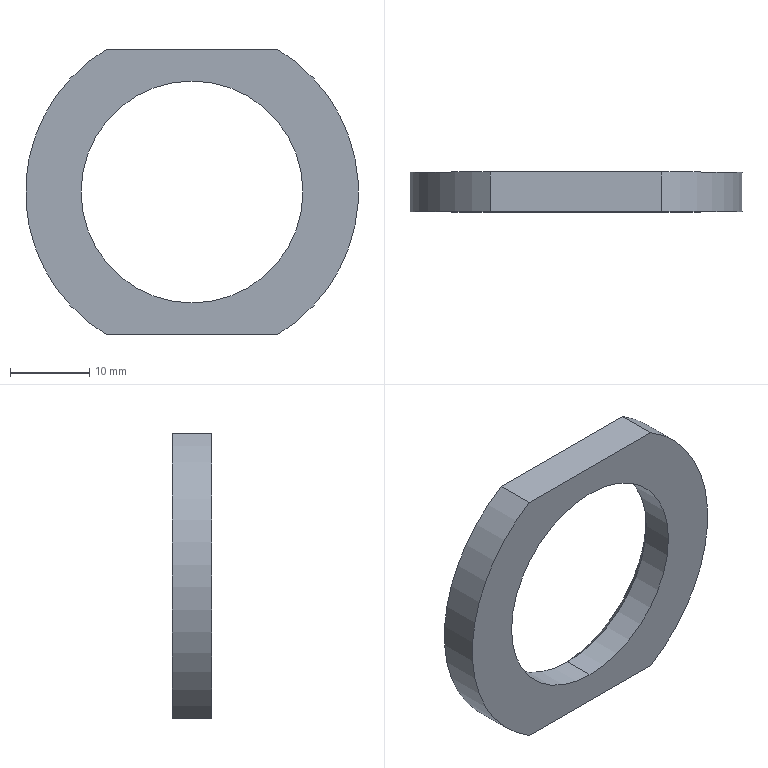Part | SolidWorks | features Extrusion 1, HoleWzd 1 | 1 solid | 10 faces | box 42 x 5 x 36 mm | volume 3362 mm3 | cylinder 4 | plane 4 | cone 2 | commonest cylinder face diameters 28 x2 42 x2
STEP:
#1=CARTESIAN_POINT('',(0.,3.975,-14.));
#2=VERTEX_POINT('',#1);
#3=CARTESIAN_POINT('',(0.,3.975,14.));
#4=VERTEX_POINT('',#3);
#5=CARTESIAN_POINT('',(0.,3.975,0.));
#6=DIRECTION('',(0.,1.,0.));
#7=DIRECTION('',(0.,0.,1.));
#8=AXIS2_PLACEMENT_3D('',#5,#6,#7);
#9=CIRCLE('',#8,14.);
#10=EDGE_CURVE('',#2,#4,#9,.T.);
#11=ORIENTED_EDGE('',*,*,#10,.F.);
#12=CARTESIAN_POINT('',(0.,5.,-15.025));
#13=VERTEX_POINT('',#12);
#14=CARTESIAN_POINT('',(0.,5.,-15.025));
#15=DIRECTION('',(0.,0.7071,-0.7071));
#16=VECTOR('',#15,1000.);
#17=LINE('',#14,#16);
#18=EDGE_CURVE('',#2,#13,#17,.T.);
#19=ORIENTED_EDGE('',*,*,#18,.T.);
#20=CARTESIAN_POINT('',(0.,5.,15.025));
#21=VERTEX_POINT('',#20);
#22=CARTESIAN_POINT('',(0.,5.,0.));
#23=DIRECTION('',(0.,1.,0.));
#24=DIRECTION('',(0.,0.,1.));
#25=AXIS2_PLACEMENT_3D('',#22,#23,#24);
#26=CIRCLE('',#25,15.025);
#27=EDGE_CURVE('',#13,#21,#26,.T.);
#28=ORIENTED_EDGE('',*,*,#27,.T.);
#29=CARTESIAN_POINT('',(0.,5.,15.025));
#30=DIRECTION('',(0.,0.7071,0.7071));
#31=VECTOR('',#30,1000.);
#32=LINE('',#29,#31);
#33=EDGE_CURVE('',#4,#21,#32,.T.);
#34=ORIENTED_EDGE('',*,*,#33,.F.);
#35=EDGE_LOOP('',(#11,#19,#28,#34));
#36=FACE_OUTER_BOUND('',#35,.T.);
#37=CARTESIAN_POINT('',(0.,5.,0.));
#38=DIRECTION('',(0.,1.,0.));
#39=DIRECTION('',(0.,0.,1.));
#40=AXIS2_PLACEMENT_3D('',#37,#38,#39);
#41=CONICAL_SURFACE('',#40,15.025,0.7854);
#42=ADVANCED_FACE('',(#36),#41,.F.);
#43=CARTESIAN_POINT('',(0.,0.,-14.));
#44=VERTEX_POINT('',#43);
#45=CARTESIAN_POINT('',(0.,0.,14.));
#46=VERTEX_POINT('',#45);
#47=CARTESIAN_POINT('',(0.,0.,0.));
#48=DIRECTION('',(0.,1.,0.));
#49=DIRECTION('',(0.,0.,1.));
#50=AXIS2_PLACEMENT_3D('',#47,#48,#49);
#51=CIRCLE('',#50,14.);
#52=EDGE_CURVE('',#44,#46,#51,.T.);
#53=ORIENTED_EDGE('',*,*,#52,.F.);
#54=CARTESIAN_POINT('',(0.,5.,-14.));
#55=DIRECTION('',(0.,1.,0.));
#56=VECTOR('',#55,1000.);
#57=LINE('',#54,#56);
#58=EDGE_CURVE('',#44,#2,#57,.T.);
#59=ORIENTED_EDGE('',*,*,#58,.T.);
#60=ORIENTED_EDGE('',*,*,#10,.T.);
#61=CARTESIAN_POINT('',(0.,5.,14.));
#62=DIRECTION('',(0.,1.,0.));
#63=VECTOR('',#62,1000.);
#64=LINE('',#61,#63);
#65=EDGE_CURVE('',#46,#4,#64,.T.);
#66=ORIENTED_EDGE('',*,*,#65,.F.);
#67=EDGE_LOOP('',(#53,#59,#60,#66));
#68=FACE_OUTER_BOUND('',#67,.T.);
#69=CARTESIAN_POINT('',(0.,5.,0.));
#70=DIRECTION('',(0.,1.,0.));
#71=DIRECTION('',(0.,0.,1.));
#72=AXIS2_PLACEMENT_3D('',#69,#70,#71);
#73=CYLINDRICAL_SURFACE('',#72,14.);
#74=ADVANCED_FACE('',(#68),#73,.F.);
#75=CARTESIAN_POINT('',(-10.817,0.,18.));
#76=VERTEX_POINT('',#75);
#77=CARTESIAN_POINT('',(10.817,0.,18.));
#78=VERTEX_POINT('',#77);
#79=CARTESIAN_POINT('',(0.,0.,18.));
#80=DIRECTION('',(1.,0.,0.));
#81=VECTOR('',#80,1000.);
#82=LINE('',#79,#81);
#83=EDGE_CURVE('',#76,#78,#82,.T.);
#84=ORIENTED_EDGE('',*,*,#83,.T.);
#85=CARTESIAN_POINT('',(10.817,5.,18.));
#86=VERTEX_POINT('',#85);
#87=CARTESIAN_POINT('',(10.817,5.,18.));
#88=DIRECTION('',(0.,-1.,0.));
#89=VECTOR('',#88,1000.);
#90=LINE('',#87,#89);
#91=EDGE_CURVE('',#86,#78,#90,.T.);
#92=ORIENTED_EDGE('',*,*,#91,.F.);
#93=CARTESIAN_POINT('',(-10.817,5.,18.));
#94=VERTEX_POINT('',#93);
#95=CARTESIAN_POINT('',(0.,5.,18.));
#96=DIRECTION('',(1.,0.,0.));
#97=VECTOR('',#96,1000.);
#98=LINE('',#95,#97);
#99=EDGE_CURVE('',#94,#86,#98,.T.);
#100=ORIENTED_EDGE('',*,*,#99,.F.);
#101=CARTESIAN_POINT('',(-10.817,5.,18.));
#102=DIRECTION('',(0.,-1.,0.));
#103=VECTOR('',#102,1000.);
#104=LINE('',#101,#103);
#105=EDGE_CURVE('',#94,#76,#104,.T.);
#106=ORIENTED_EDGE('',*,*,#105,.T.);
#107=EDGE_LOOP('',(#84,#92,#100,#106));
#108=FACE_OUTER_BOUND('',#107,.T.);
#109=CARTESIAN_POINT('',(0.,5.,18.));
#110=DIRECTION('',(0.,0.,-1.));
#111=DIRECTION('',(-1.,0.,0.));
#112=AXIS2_PLACEMENT_3D('',#109,#110,#111);
#113=PLANE('',#112);
#114=ADVANCED_FACE('',(#108),#113,.F.);
#115=CARTESIAN_POINT('',(10.817,0.,-18.));
#116=VERTEX_POINT('',#115);
#117=CARTESIAN_POINT('',(0.,0.,0.));
#118=DIRECTION('',(0.,1.,0.));
#119=DIRECTION('',(0.,0.,1.));
#120=AXIS2_PLACEMENT_3D('',#117,#118,#119);
#121=CIRCLE('',#120,21.);
#122=EDGE_CURVE('',#78,#116,#121,.T.);
#123=ORIENTED_EDGE('',*,*,#122,.T.);
#124=CARTESIAN_POINT('',(10.817,5.,-18.));
#125=VERTEX_POINT('',#124);
#126=CARTESIAN_POINT('',(10.817,5.,-18.));
#127=DIRECTION('',(0.,-1.,0.));
#128=VECTOR('',#127,1000.);
#129=LINE('',#126,#128);
#130=EDGE_CURVE('',#125,#116,#129,.T.);
#131=ORIENTED_EDGE('',*,*,#130,.F.);
#132=CARTESIAN_POINT('',(0.,5.,0.));
#133=DIRECTION('',(0.,1.,0.));
#134=DIRECTION('',(0.,0.,1.));
#135=AXIS2_PLACEMENT_3D('',#132,#133,#134);
#136=CIRCLE('',#135,21.);
#137=EDGE_CURVE('',#86,#125,#136,.T.);
#138=ORIENTED_EDGE('',*,*,#137,.F.);
#139=ORIENTED_EDGE('',*,*,#91,.T.);
#140=EDGE_LOOP('',(#123,#131,#138,#139));
#141=FACE_OUTER_BOUND('',#140,.T.);
#142=CARTESIAN_POINT('',(0.,5.,0.));
#143=DIRECTION('',(0.,-1.,0.));
#144=DIRECTION('',(0.,0.,-1.));
#145=AXIS2_PLACEMENT_3D('',#142,#143,#144);
#146=CYLINDRICAL_SURFACE('',#145,21.);
#147=ADVANCED_FACE('',(#141),#146,.T.);
#148=CARTESIAN_POINT('',(-10.817,0.,-18.));
#149=VERTEX_POINT('',#148);
#150=CARTESIAN_POINT('',(0.,0.,-18.));
#151=DIRECTION('',(1.,0.,0.));
#152=VECTOR('',#151,1000.);
#153=LINE('',#150,#152);
#154=EDGE_CURVE('',#149,#116,#153,.T.);
#155=ORIENTED_EDGE('',*,*,#154,.F.);
#156=CARTESIAN_POINT('',(-10.817,5.,-18.));
#157=VERTEX_POINT('',#156);
#158=CARTESIAN_POINT('',(-10.817,5.,-18.));
#159=DIRECTION('',(0.,-1.,0.));
#160=VECTOR('',#159,1000.);
#161=LINE('',#158,#160);
#162=EDGE_CURVE('',#157,#149,#161,.T.);
#163=ORIENTED_EDGE('',*,*,#162,.F.);
#164=CARTESIAN_POINT('',(0.,5.,-18.));
#165=DIRECTION('',(1.,0.,0.));
#166=VECTOR('',#165,1000.);
#167=LINE('',#164,#166);
#168=EDGE_CURVE('',#157,#125,#167,.T.);
#169=ORIENTED_EDGE('',*,*,#168,.T.);
#170=ORIENTED_EDGE('',*,*,#130,.T.);
#171=EDGE_LOOP('',(#155,#163,#169,#170));
#172=FACE_OUTER_BOUND('',#171,.T.);
#173=CARTESIAN_POINT('',(0.,5.,-18.));
#174=DIRECTION('',(0.,0.,-1.));
#175=DIRECTION('',(-1.,0.,0.));
#176=AXIS2_PLACEMENT_3D('',#173,#174,#175);
#177=PLANE('',#176);
#178=ADVANCED_FACE('',(#172),#177,.T.);
#179=CARTESIAN_POINT('',(0.,0.,0.));
#180=DIRECTION('',(0.,1.,0.));
#181=DIRECTION('',(0.,0.,1.));
#182=AXIS2_PLACEMENT_3D('',#179,#180,#181);
#183=CIRCLE('',#182,21.);
#184=EDGE_CURVE('',#149,#76,#183,.T.);
#185=ORIENTED_EDGE('',*,*,#184,.T.);
#186=ORIENTED_EDGE('',*,*,#105,.F.);
#187=CARTESIAN_POINT('',(0.,5.,0.));
#188=DIRECTION('',(0.,1.,0.));
#189=DIRECTION('',(0.,0.,1.));
#190=AXIS2_PLACEMENT_3D('',#187,#188,#189);
#191=CIRCLE('',#190,21.);
#192=EDGE_CURVE('',#157,#94,#191,.T.);
#193=ORIENTED_EDGE('',*,*,#192,.F.);
#194=ORIENTED_EDGE('',*,*,#162,.T.);
#195=EDGE_LOOP('',(#185,#186,#193,#194));
#196=FACE_OUTER_BOUND('',#195,.T.);
#197=CARTESIAN_POINT('',(0.,5.,0.));
#198=DIRECTION('',(0.,-1.,0.));
#199=DIRECTION('',(0.,0.,-1.));
#200=AXIS2_PLACEMENT_3D('',#197,#198,#199);
#201=CYLINDRICAL_SURFACE('',#200,21.);
#202=ADVANCED_FACE('',(#196),#201,.T.);
#203=CARTESIAN_POINT('',(0.,5.,0.));
#204=DIRECTION('',(0.,1.,0.));
#205=DIRECTION('',(0.,0.,1.));
#206=AXIS2_PLACEMENT_3D('',#203,#204,#205);
#207=CIRCLE('',#206,15.025);
#208=EDGE_CURVE('',#21,#13,#207,.T.);
#209=ORIENTED_EDGE('',*,*,#208,.F.);
#210=ORIENTED_EDGE('',*,*,#27,.F.);
#211=EDGE_LOOP('',(#209,#210));
#212=FACE_BOUND('',#211,.T.);
#213=ORIENTED_EDGE('',*,*,#99,.T.);
#214=ORIENTED_EDGE('',*,*,#137,.T.);
#215=ORIENTED_EDGE('',*,*,#168,.F.);
#216=ORIENTED_EDGE('',*,*,#192,.T.);
#217=EDGE_LOOP('',(#213,#214,#215,#216));
#218=FACE_OUTER_BOUND('',#217,.T.);
#219=CARTESIAN_POINT('',(0.,5.,0.));
#220=DIRECTION('',(0.,1.,0.));
#221=DIRECTION('',(0.,0.,1.));
#222=AXIS2_PLACEMENT_3D('',#219,#220,#221);
#223=PLANE('',#222);
#224=ADVANCED_FACE('',(#212,#218),#223,.T.);
#225=CARTESIAN_POINT('',(0.,0.,0.));
#226=DIRECTION('',(0.,1.,0.));
#227=DIRECTION('',(0.,0.,1.));
#228=AXIS2_PLACEMENT_3D('',#225,#226,#227);
#229=CIRCLE('',#228,14.);
#230=EDGE_CURVE('',#46,#44,#229,.T.);
#231=ORIENTED_EDGE('',*,*,#230,.T.);
#232=ORIENTED_EDGE('',*,*,#52,.T.);
#233=EDGE_LOOP('',(#231,#232));
#234=FACE_BOUND('',#233,.T.);
#235=ORIENTED_EDGE('',*,*,#83,.F.);
#236=ORIENTED_EDGE('',*,*,#184,.F.);
#237=ORIENTED_EDGE('',*,*,#154,.T.);
#238=ORIENTED_EDGE('',*,*,#122,.F.);
#239=EDGE_LOOP('',(#235,#236,#237,#238));
#240=FACE_OUTER_BOUND('',#239,.T.);
#241=CARTESIAN_POINT('',(0.,0.,0.));
#242=DIRECTION('',(0.,1.,0.));
#243=DIRECTION('',(0.,0.,1.));
#244=AXIS2_PLACEMENT_3D('',#241,#242,#243);
#245=PLANE('',#244);
#246=ADVANCED_FACE('',(#234,#240),#245,.F.);
#247=ORIENTED_EDGE('',*,*,#58,.F.);
#248=ORIENTED_EDGE('',*,*,#230,.F.);
#249=ORIENTED_EDGE('',*,*,#65,.T.);
#250=CARTESIAN_POINT('',(0.,3.975,0.));
#251=DIRECTION('',(0.,1.,0.));
#252=DIRECTION('',(0.,0.,1.));
#253=AXIS2_PLACEMENT_3D('',#250,#251,#252);
#254=CIRCLE('',#253,14.);
#255=EDGE_CURVE('',#4,#2,#254,.T.);
#256=ORIENTED_EDGE('',*,*,#255,.T.);
#257=EDGE_LOOP('',(#247,#248,#249,#256));
#258=FACE_OUTER_BOUND('',#257,.T.);
#259=CARTESIAN_POINT('',(0.,5.,0.));
#260=DIRECTION('',(0.,1.,0.));
#261=DIRECTION('',(0.,0.,1.));
#262=AXIS2_PLACEMENT_3D('',#259,#260,#261);
#263=CYLINDRICAL_SURFACE('',#262,14.);
#264=ADVANCED_FACE('',(#258),#263,.F.);
#265=ORIENTED_EDGE('',*,*,#18,.F.);
#266=ORIENTED_EDGE('',*,*,#255,.F.);
#267=ORIENTED_EDGE('',*,*,#33,.T.);
#268=ORIENTED_EDGE('',*,*,#208,.T.);
#269=EDGE_LOOP('',(#265,#266,#267,#268));
#270=FACE_OUTER_BOUND('',#269,.T.);
#271=CARTESIAN_POINT('',(0.,5.,0.));
#272=DIRECTION('',(0.,1.,0.));
#273=DIRECTION('',(0.,0.,1.));
#274=AXIS2_PLACEMENT_3D('',#271,#272,#273);
#275=CONICAL_SURFACE('',#274,15.025,0.7854);
#276=ADVANCED_FACE('',(#270),#275,.F.);
#277=CLOSED_SHELL('',(#42,#74,#114,#147,#178,#202,#224,#246,#264,#276));
#278=MANIFOLD_SOLID_BREP('',#277);
#279=CARTESIAN_POINT('',(0.,0.,0.));
#280=DIRECTION('',(0.,0.,1.));
#281=DIRECTION('',(1.,0.,0.));
#282=AXIS2_PLACEMENT_3D('',#279,#280,#281);
#283=(LENGTH_UNIT()NAMED_UNIT(*)SI_UNIT(.MILLI.,.METRE.));
#284=UNCERTAINTY_MEASURE_WITH_UNIT(LENGTH_MEASURE(0.00001),#283,'','');
#285=(NAMED_UNIT(*)PLANE_ANGLE_UNIT()SI_UNIT($,.RADIAN.));
#286=(NAMED_UNIT(*)SI_UNIT($,.STERADIAN.)SOLID_ANGLE_UNIT());
#287=(GEOMETRIC_REPRESENTATION_CONTEXT(3)GLOBAL_UNCERTAINTY_ASSIGNED_CONTEXT((#284))GLOBAL_UNIT_ASSIGNED_CONTEXT((#283,#285,#286))REPRESENTATION_CONTEXT('',''));
#288=ADVANCED_BREP_SHAPE_REPRESENTATION('',(#278,#282),#287);